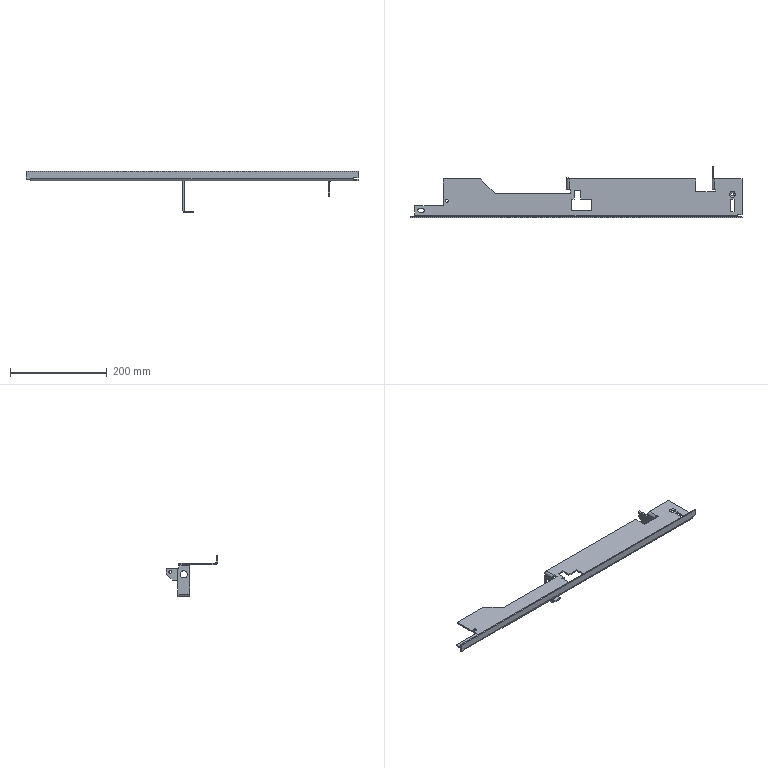Part | STEP file | Right guide rail PN_0062 | 1 solid | 78 faces | box 686 x 106 x 85 mm | volume 168135 mm3 | plane 55 | cylinder 21 | cone 2 | commonest cylinder face diameters 4.2 x4 6 x4 10.2 x4 15 x4 7 x3 6.8 x2